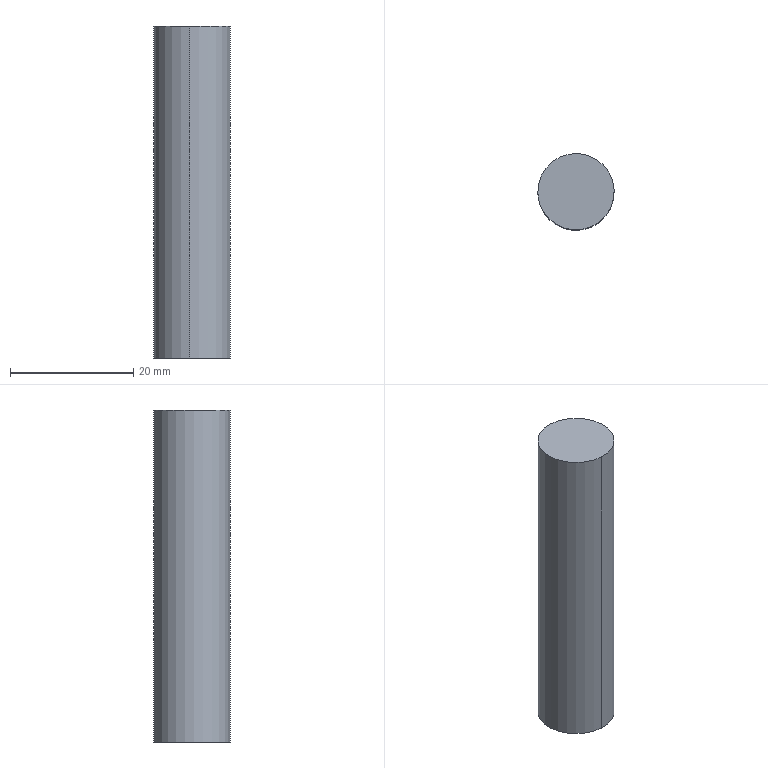Part | STEP file | 1_id902_x_t | 1 solid | 4 faces | box 12.423 x 12.423 x 53.975 mm | volume 6543 mm3 | cylinder 2 | plane 2 | commonest cylinder face diameters 12.423 x2
STEP:
#1=CARTESIAN_POINT('',(0.,0.,0.));
#2=DIRECTION('',(0.,0.,1.));
#3=DIRECTION('',(1.,0.,0.));
#4=AXIS2_PLACEMENT_3D('',#1,#2,#3);
#5=CARTESIAN_POINT('',(976.519,332.83,-107.411));
#6=VERTEX_POINT('',#5);
#7=CARTESIAN_POINT('',(976.519,332.83,-53.436));
#8=VERTEX_POINT('',#7);
#9=CARTESIAN_POINT('',(976.519,332.83,-107.411));
#10=DIRECTION('',(0.,0.,1.));
#11=VECTOR('',#10,1.);
#12=LINE('',#9,#11);
#13=CARTESIAN_POINT('',(976.138,326.63,-120.111));
#14=DIRECTION('',(0.,0.,1.));
#15=DIRECTION('',(-0.06122,-0.9981,0.));
#16=AXIS2_PLACEMENT_3D('',#13,#14,#15);
#17=CYLINDRICAL_SURFACE('',#16,6.212);
#18=CARTESIAN_POINT('',(3.142,12.7));
#19=DIRECTION('',(0.,1.));
#20=VECTOR('',#19,1.);
#21=LINE('',#18,#20);
#22=(GEOMETRIC_REPRESENTATION_CONTEXT(2)PARAMETRIC_REPRESENTATION_CONTEXT()REPRESENTATION_CONTEXT('',''));
#23=DEFINITIONAL_REPRESENTATION('',(#21),#22);
#24=PCURVE('',#17,#23);
#25=CARTESIAN_POINT('',(976.138,326.63,-120.111));
#26=DIRECTION('',(0.,0.,1.));
#27=DIRECTION('',(-0.06122,-0.9981,0.));
#28=AXIS2_PLACEMENT_3D('',#25,#26,#27);
#29=CYLINDRICAL_SURFACE('',#28,6.212);
#30=CARTESIAN_POINT('',(3.142,12.7));
#31=DIRECTION('',(0.,1.));
#32=VECTOR('',#31,1.);
#33=LINE('',#30,#32);
#34=(GEOMETRIC_REPRESENTATION_CONTEXT(2)PARAMETRIC_REPRESENTATION_CONTEXT()REPRESENTATION_CONTEXT('',''));
#35=DEFINITIONAL_REPRESENTATION('',(#33),#34);
#36=PCURVE('',#29,#35);
#37=SURFACE_CURVE('',#12,(#24,#36),.PCURVE_S1.);
#38=EDGE_CURVE('',#6,#8,#37,.T.);
#39=ORIENTED_EDGE('',*,*,#38,.F.);
#40=CARTESIAN_POINT('',(975.758,320.43,-107.411));
#41=VERTEX_POINT('',#40);
#42=CARTESIAN_POINT('',(976.138,326.63,-107.411));
#43=DIRECTION('',(0.,0.,-1.));
#44=DIRECTION('',(-0.06122,-0.9981,0.));
#45=AXIS2_PLACEMENT_3D('',#42,#43,#44);
#46=CIRCLE('',#45,6.212);
#47=CARTESIAN_POINT('',(6.283,12.7));
#48=DIRECTION('',(-1.,0.));
#49=VECTOR('',#48,1.);
#50=LINE('',#47,#49);
#51=(GEOMETRIC_REPRESENTATION_CONTEXT(2)PARAMETRIC_REPRESENTATION_CONTEXT()REPRESENTATION_CONTEXT('',''));
#52=DEFINITIONAL_REPRESENTATION('',(#50),#51);
#53=PCURVE('',#17,#52);
#54=CARTESIAN_POINT('',(976.138,326.63,-107.411));
#55=DIRECTION('',(0.,0.,-1.));
#56=DIRECTION('',(0.8435,0.5372,0.));
#57=AXIS2_PLACEMENT_3D('',#54,#55,#56);
#58=PLANE('',#57);
#59=CARTESIAN_POINT('',(0.,0.));
#60=DIRECTION('',(-0.5878,0.809));
#61=AXIS2_PLACEMENT_2D('',#59,#60);
#62=CIRCLE('',#61,6.212);
#63=(GEOMETRIC_REPRESENTATION_CONTEXT(2)PARAMETRIC_REPRESENTATION_CONTEXT()REPRESENTATION_CONTEXT('',''));
#64=DEFINITIONAL_REPRESENTATION('',(#62),#63);
#65=PCURVE('',#58,#64);
#66=SURFACE_CURVE('',#46,(#53,#65),.PCURVE_S1.);
#67=EDGE_CURVE('',#41,#6,#66,.T.);
#68=ORIENTED_EDGE('',*,*,#67,.F.);
#69=CARTESIAN_POINT('',(975.758,320.43,-53.436));
#70=VERTEX_POINT('',#69);
#71=CARTESIAN_POINT('',(975.758,320.43,-107.411));
#72=DIRECTION('',(0.,0.,-1.));
#73=VECTOR('',#72,1.);
#74=LINE('',#71,#73);
#75=CARTESIAN_POINT('',(6.283,12.7));
#76=DIRECTION('',(0.,-1.));
#77=VECTOR('',#76,1.);
#78=LINE('',#75,#77);
#79=(GEOMETRIC_REPRESENTATION_CONTEXT(2)PARAMETRIC_REPRESENTATION_CONTEXT()REPRESENTATION_CONTEXT('',''));
#80=DEFINITIONAL_REPRESENTATION('',(#78),#79);
#81=PCURVE('',#17,#80);
#82=CARTESIAN_POINT('',(0.,12.7));
#83=DIRECTION('',(0.,-1.));
#84=VECTOR('',#83,1.);
#85=LINE('',#82,#84);
#86=(GEOMETRIC_REPRESENTATION_CONTEXT(2)PARAMETRIC_REPRESENTATION_CONTEXT()REPRESENTATION_CONTEXT('',''));
#87=DEFINITIONAL_REPRESENTATION('',(#85),#86);
#88=PCURVE('',#29,#87);
#89=SURFACE_CURVE('',#74,(#81,#88),.PCURVE_S1.);
#90=EDGE_CURVE('',#70,#41,#89,.T.);
#91=ORIENTED_EDGE('',*,*,#90,.F.);
#92=CARTESIAN_POINT('',(976.138,326.63,-53.436));
#93=DIRECTION('',(0.,0.,1.));
#94=DIRECTION('',(0.06122,0.9981,0.));
#95=AXIS2_PLACEMENT_3D('',#92,#93,#94);
#96=CIRCLE('',#95,6.212);
#97=CARTESIAN_POINT('',(3.142,66.675));
#98=DIRECTION('',(1.,0.));
#99=VECTOR('',#98,1.);
#100=LINE('',#97,#99);
#101=(GEOMETRIC_REPRESENTATION_CONTEXT(2)PARAMETRIC_REPRESENTATION_CONTEXT()REPRESENTATION_CONTEXT('',''));
#102=DEFINITIONAL_REPRESENTATION('',(#100),#101);
#103=PCURVE('',#17,#102);
#104=CARTESIAN_POINT('',(976.138,326.63,-53.436));
#105=DIRECTION('',(0.,0.,1.));
#106=DIRECTION('',(-0.5372,0.8435,0.));
#107=AXIS2_PLACEMENT_3D('',#104,#105,#106);
#108=PLANE('',#107);
#109=CARTESIAN_POINT('',(0.,0.));
#110=DIRECTION('',(0.809,-0.5878));
#111=AXIS2_PLACEMENT_2D('',#109,#110);
#112=CIRCLE('',#111,6.212);
#113=(GEOMETRIC_REPRESENTATION_CONTEXT(2)PARAMETRIC_REPRESENTATION_CONTEXT()REPRESENTATION_CONTEXT('',''));
#114=DEFINITIONAL_REPRESENTATION('',(#112),#113);
#115=PCURVE('',#108,#114);
#116=SURFACE_CURVE('',#96,(#103,#115),.PCURVE_S1.);
#117=EDGE_CURVE('',#8,#70,#116,.T.);
#118=ORIENTED_EDGE('',*,*,#117,.F.);
#119=EDGE_LOOP('',(#39,#68,#91,#118));
#120=FACE_BOUND('',#119,.T.);
#121=ADVANCED_FACE('',(#120),#17,.T.);
#122=ORIENTED_EDGE('',*,*,#117,.T.);
#123=CARTESIAN_POINT('',(976.138,326.63,-53.436));
#124=DIRECTION('',(0.,0.,1.));
#125=DIRECTION('',(-0.06122,-0.9981,0.));
#126=AXIS2_PLACEMENT_3D('',#123,#124,#125);
#127=CIRCLE('',#126,6.212);
#128=CARTESIAN_POINT('',(0.,0.));
#129=DIRECTION('',(-0.809,0.5878));
#130=AXIS2_PLACEMENT_2D('',#128,#129);
#131=CIRCLE('',#130,6.212);
#132=(GEOMETRIC_REPRESENTATION_CONTEXT(2)PARAMETRIC_REPRESENTATION_CONTEXT()REPRESENTATION_CONTEXT('',''));
#133=DEFINITIONAL_REPRESENTATION('',(#131),#132);
#134=PCURVE('',#108,#133);
#135=CARTESIAN_POINT('',(0.,66.675));
#136=DIRECTION('',(1.,0.));
#137=VECTOR('',#136,1.);
#138=LINE('',#135,#137);
#139=(GEOMETRIC_REPRESENTATION_CONTEXT(2)PARAMETRIC_REPRESENTATION_CONTEXT()REPRESENTATION_CONTEXT('',''));
#140=DEFINITIONAL_REPRESENTATION('',(#138),#139);
#141=PCURVE('',#29,#140);
#142=SURFACE_CURVE('',#127,(#134,#141),.PCURVE_S1.);
#143=EDGE_CURVE('',#70,#8,#142,.T.);
#144=ORIENTED_EDGE('',*,*,#143,.T.);
#145=EDGE_LOOP('',(#122,#144));
#146=FACE_BOUND('',#145,.T.);
#147=ADVANCED_FACE('',(#146),#108,.T.);
#148=ORIENTED_EDGE('',*,*,#90,.T.);
#149=CARTESIAN_POINT('',(976.138,326.63,-107.411));
#150=DIRECTION('',(0.,0.,-1.));
#151=DIRECTION('',(0.06122,0.9981,0.));
#152=AXIS2_PLACEMENT_3D('',#149,#150,#151);
#153=CIRCLE('',#152,6.212);
#154=CARTESIAN_POINT('',(3.142,12.7));
#155=DIRECTION('',(-1.,0.));
#156=VECTOR('',#155,1.);
#157=LINE('',#154,#156);
#158=(GEOMETRIC_REPRESENTATION_CONTEXT(2)PARAMETRIC_REPRESENTATION_CONTEXT()REPRESENTATION_CONTEXT('',''));
#159=DEFINITIONAL_REPRESENTATION('',(#157),#158);
#160=PCURVE('',#29,#159);
#161=CARTESIAN_POINT('',(0.,0.));
#162=DIRECTION('',(0.5878,-0.809));
#163=AXIS2_PLACEMENT_2D('',#161,#162);
#164=CIRCLE('',#163,6.212);
#165=(GEOMETRIC_REPRESENTATION_CONTEXT(2)PARAMETRIC_REPRESENTATION_CONTEXT()REPRESENTATION_CONTEXT('',''));
#166=DEFINITIONAL_REPRESENTATION('',(#164),#165);
#167=PCURVE('',#58,#166);
#168=SURFACE_CURVE('',#153,(#160,#167),.PCURVE_S1.);
#169=EDGE_CURVE('',#6,#41,#168,.T.);
#170=ORIENTED_EDGE('',*,*,#169,.F.);
#171=ORIENTED_EDGE('',*,*,#38,.T.);
#172=ORIENTED_EDGE('',*,*,#143,.F.);
#173=EDGE_LOOP('',(#148,#170,#171,#172));
#174=FACE_BOUND('',#173,.T.);
#175=ADVANCED_FACE('',(#174),#29,.T.);
#176=ORIENTED_EDGE('',*,*,#169,.T.);
#177=ORIENTED_EDGE('',*,*,#67,.T.);
#178=EDGE_LOOP('',(#176,#177));
#179=FACE_BOUND('',#178,.T.);
#180=ADVANCED_FACE('',(#179),#58,.T.);
#181=CLOSED_SHELL('',(#121,#147,#175,#180));
#182=MANIFOLD_SOLID_BREP('',#181);
#183=(LENGTH_UNIT()NAMED_UNIT(*)SI_UNIT(.MILLI.,.METRE.));
#184=UNCERTAINTY_MEASURE_WITH_UNIT(LENGTH_MEASURE(0.0000001),#183,'','');
#185=(NAMED_UNIT(*)PLANE_ANGLE_UNIT()SI_UNIT($,.RADIAN.));
#186=(NAMED_UNIT(*)SI_UNIT($,.STERADIAN.)SOLID_ANGLE_UNIT());
#187=(GEOMETRIC_REPRESENTATION_CONTEXT(3)GLOBAL_UNCERTAINTY_ASSIGNED_CONTEXT((#184))GLOBAL_UNIT_ASSIGNED_CONTEXT((#183,#185,#186))REPRESENTATION_CONTEXT('',''));
#188=ADVANCED_BREP_SHAPE_REPRESENTATION('',(#4,#182),#187);